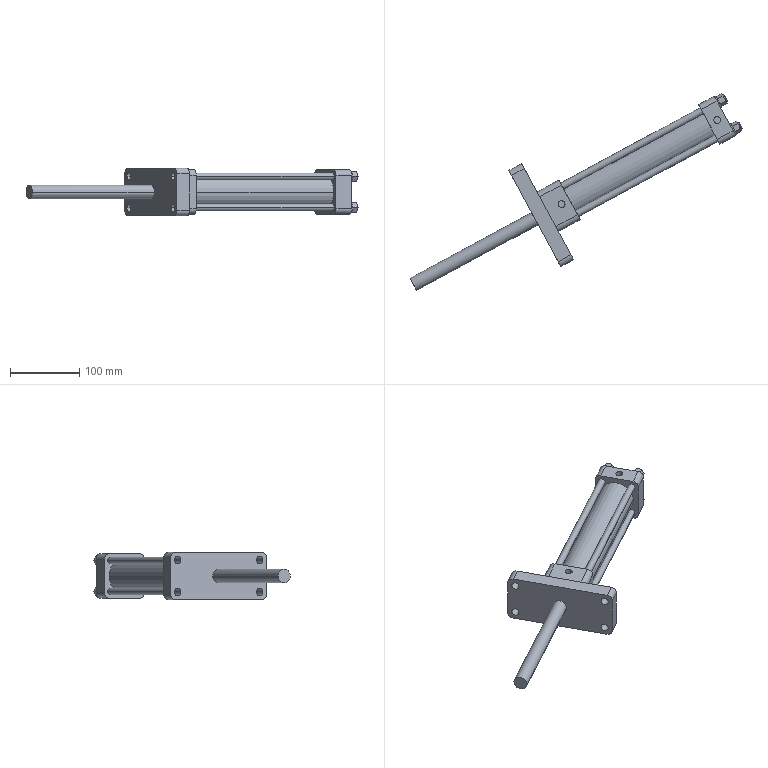Part | Creo | 1 solid | 108 faces | box 480.645 x 284.693 x 69 mm | volume 1068711 mm3 | plane 56 | cylinder 52 | commonest cylinder face diameters 10 x20 16 x12 11 x8 18 x8 20 x2 50 x2